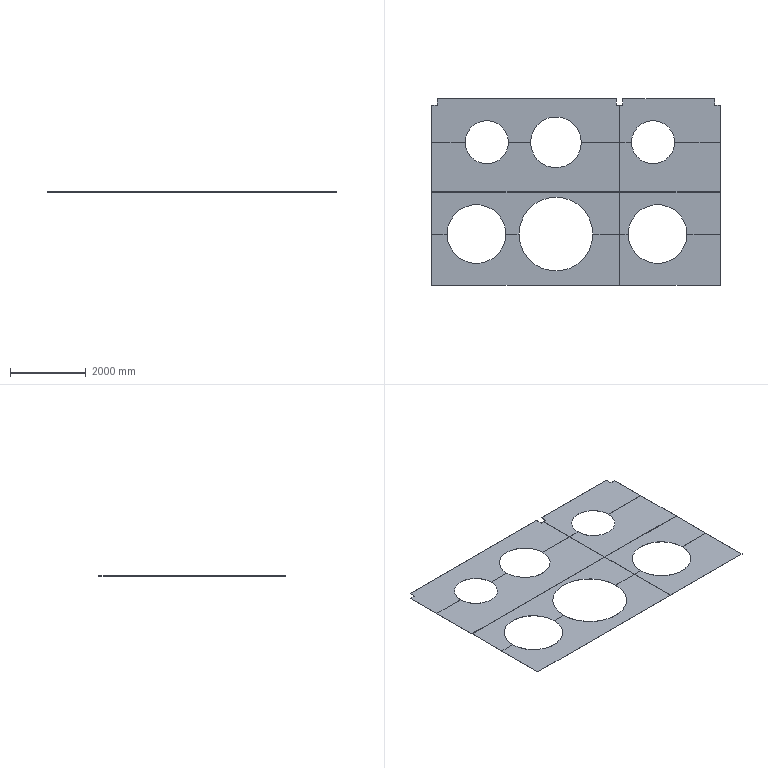Part | STEP file | 粉仓花纹Plate | 8 solids | 80 faces | box 7625 x 4925 x 3 mm | volume 81712704 mm3 | plane 68 | cylinder 12 | commonest cylinder face diameters 1140 x4 1550 x4 1340 x2 1950 x2